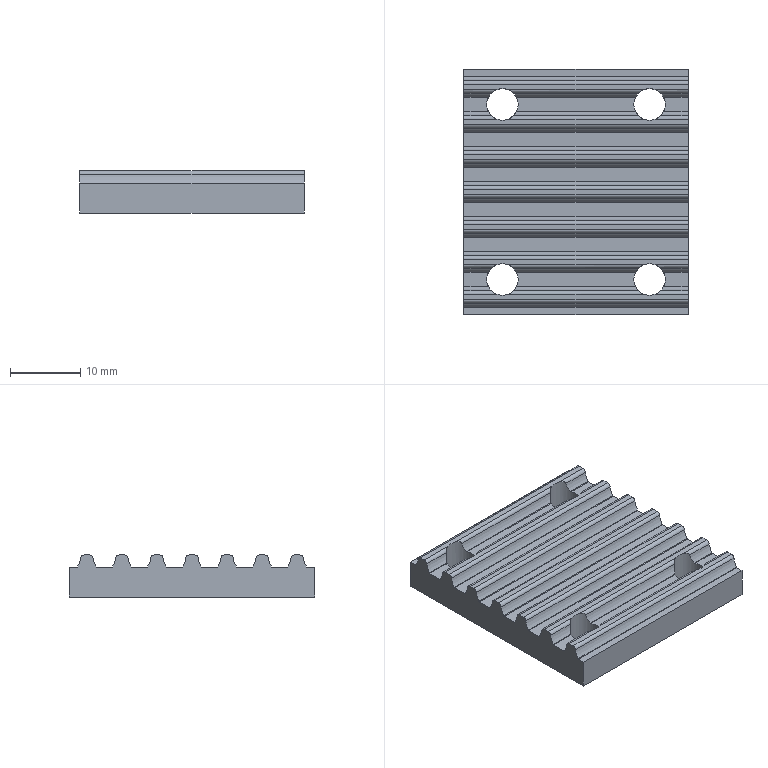Part | NX | features 5003_018_C-TBCR-S5M150 2 | 1 solid | 94 faces | box 32 x 35 x 6 mm | volume 5224 mm3 | cylinder 70 | plane 24 | commonest cylinder face diameters 0.197 x22 1 x22 6.308 x22 4.5 x4